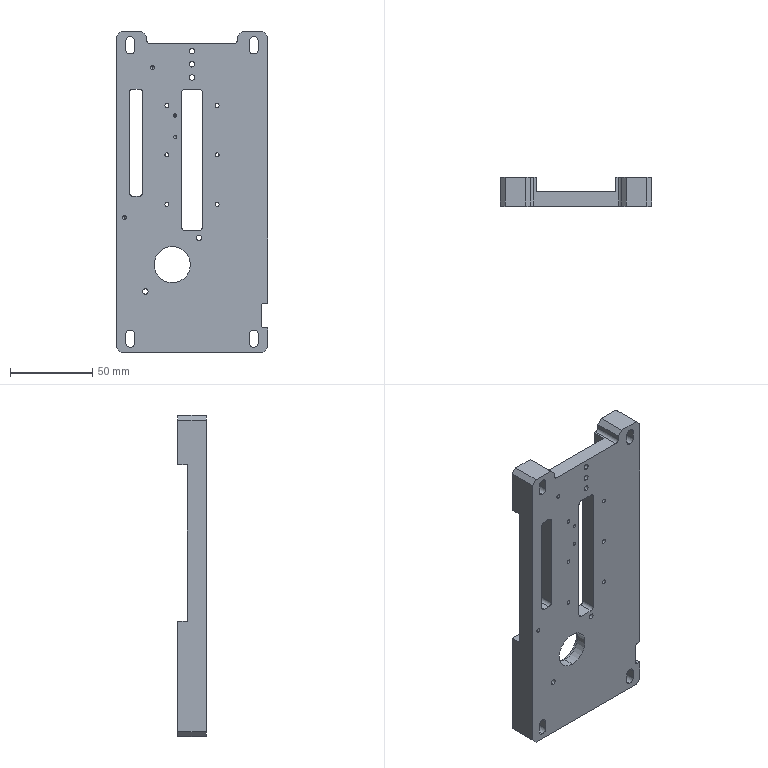Part | SolidWorks | features ICE 10, HoleWzd 7, Cut 4, Fillet 4, 3DProfileFeature 3, Chamfer 3, Extrusion 1, LPattern 1 | 1 solid | 127 faces | box 92 x 17.5 x 195 mm | volume 172587 mm3 | cylinder 62 | plane 53 | cone 12 | commonest cylinder face diameters 2.5 x16 3.3 x14 4 x12 5.5 x12 2.05 x4 22 x2